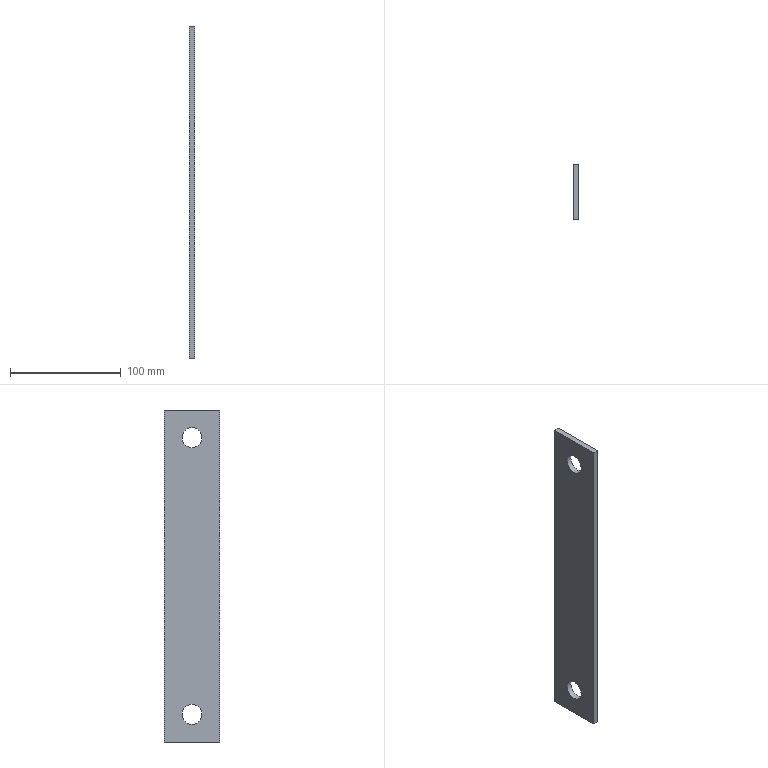Part | NX | features solid 2 | 1 solid | 8 faces | box 5 x 50 x 300 mm | volume 72455 mm3 | plane 6 | cylinder 2 | commonest cylinder face diameters 18 x2
STEP:
#1=CARTESIAN_POINT('',(700.,395.,165.));
#2=VERTEX_POINT('',#1);
#3=CARTESIAN_POINT('',(705.,395.,165.));
#4=VERTEX_POINT('',#3);
#5=CARTESIAN_POINT('',(690.,395.,165.));
#6=DIRECTION('',(1.,0.,0.));
#7=VECTOR('',#6,1000.);
#8=LINE('',#5,#7);
#9=EDGE_CURVE('',#2,#4,#8,.T.);
#10=ORIENTED_EDGE('',*,*,#9,.F.);
#11=CARTESIAN_POINT('',(700.,345.,165.));
#12=VERTEX_POINT('',#11);
#13=CARTESIAN_POINT('',(700.,350.,165.));
#14=DIRECTION('',(0.,-1.,0.));
#15=VECTOR('',#14,1000.);
#16=LINE('',#13,#15);
#17=EDGE_CURVE('',#12,#2,#16,.F.);
#18=ORIENTED_EDGE('',*,*,#17,.F.);
#19=CARTESIAN_POINT('',(705.,345.,165.));
#20=VERTEX_POINT('',#19);
#21=CARTESIAN_POINT('',(700.,345.,165.));
#22=DIRECTION('',(-1.,0.,0.));
#23=VECTOR('',#22,1000.);
#24=LINE('',#21,#23);
#25=EDGE_CURVE('',#12,#20,#24,.F.);
#26=ORIENTED_EDGE('',*,*,#25,.T.);
#27=CARTESIAN_POINT('',(705.,350.,165.));
#28=DIRECTION('',(0.,-1.,0.));
#29=VECTOR('',#28,1000.);
#30=LINE('',#27,#29);
#31=EDGE_CURVE('',#20,#4,#30,.F.);
#32=ORIENTED_EDGE('',*,*,#31,.T.);
#33=EDGE_LOOP('',(#10,#18,#26,#32));
#34=FACE_BOUND('',#33,.T.);
#35=CARTESIAN_POINT('',(690.,350.,165.));
#36=DIRECTION('',(0.,0.,1.));
#37=DIRECTION('',(0.,1.,0.));
#38=AXIS2_PLACEMENT_3D('',#35,#36,#37);
#39=PLANE('',#38);
#40=ADVANCED_FACE('',(#34),#39,.T.);
#41=ORIENTED_EDGE('',*,*,#25,.F.);
#42=CARTESIAN_POINT('',(700.,345.,-135.));
#43=VERTEX_POINT('',#42);
#44=CARTESIAN_POINT('',(700.,345.,-35.));
#45=DIRECTION('',(0.,0.,-1.));
#46=VECTOR('',#45,1000.);
#47=LINE('',#44,#46);
#48=EDGE_CURVE('',#12,#43,#47,.T.);
#49=ORIENTED_EDGE('',*,*,#48,.T.);
#50=CARTESIAN_POINT('',(705.,345.,-135.));
#51=VERTEX_POINT('',#50);
#52=CARTESIAN_POINT('',(700.,345.,-135.));
#53=DIRECTION('',(-1.,0.,0.));
#54=VECTOR('',#53,1000.);
#55=LINE('',#52,#54);
#56=EDGE_CURVE('',#43,#51,#55,.F.);
#57=ORIENTED_EDGE('',*,*,#56,.T.);
#58=CARTESIAN_POINT('',(705.,345.,-35.));
#59=DIRECTION('',(0.,0.,1.));
#60=VECTOR('',#59,1000.);
#61=LINE('',#58,#60);
#62=EDGE_CURVE('',#20,#51,#61,.F.);
#63=ORIENTED_EDGE('',*,*,#62,.F.);
#64=EDGE_LOOP('',(#41,#49,#57,#63));
#65=FACE_BOUND('',#64,.T.);
#66=CARTESIAN_POINT('',(700.,345.,-35.));
#67=DIRECTION('',(0.,1.,0.));
#68=DIRECTION('',(0.,0.,-1.));
#69=AXIS2_PLACEMENT_3D('',#66,#67,#68);
#70=PLANE('',#69);
#71=ADVANCED_FACE('',(#65),#70,.F.);
#72=ORIENTED_EDGE('',*,*,#56,.F.);
#73=CARTESIAN_POINT('',(700.,395.,-135.));
#74=VERTEX_POINT('',#73);
#75=CARTESIAN_POINT('',(700.,345.,-135.));
#76=DIRECTION('',(0.,1.,0.));
#77=VECTOR('',#76,1000.);
#78=LINE('',#75,#77);
#79=EDGE_CURVE('',#43,#74,#78,.T.);
#80=ORIENTED_EDGE('',*,*,#79,.T.);
#81=CARTESIAN_POINT('',(705.,395.,-135.));
#82=VERTEX_POINT('',#81);
#83=CARTESIAN_POINT('',(700.,395.,-135.));
#84=DIRECTION('',(-1.,0.,0.));
#85=VECTOR('',#84,1000.);
#86=LINE('',#83,#85);
#87=EDGE_CURVE('',#74,#82,#86,.F.);
#88=ORIENTED_EDGE('',*,*,#87,.T.);
#89=CARTESIAN_POINT('',(705.,345.,-135.));
#90=DIRECTION('',(0.,1.,0.));
#91=VECTOR('',#90,1000.);
#92=LINE('',#89,#91);
#93=EDGE_CURVE('',#51,#82,#92,.T.);
#94=ORIENTED_EDGE('',*,*,#93,.F.);
#95=EDGE_LOOP('',(#72,#80,#88,#94));
#96=FACE_BOUND('',#95,.T.);
#97=CARTESIAN_POINT('',(700.,345.,-135.));
#98=DIRECTION('',(0.,0.,1.));
#99=DIRECTION('',(0.,1.,0.));
#100=AXIS2_PLACEMENT_3D('',#97,#98,#99);
#101=PLANE('',#100);
#102=ADVANCED_FACE('',(#96),#101,.F.);
#103=CARTESIAN_POINT('',(700.,395.,-35.));
#104=DIRECTION('',(0.,0.,-1.));
#105=VECTOR('',#104,1000.);
#106=LINE('',#103,#105);
#107=EDGE_CURVE('',#2,#74,#106,.T.);
#108=ORIENTED_EDGE('',*,*,#107,.F.);
#109=ORIENTED_EDGE('',*,*,#9,.T.);
#110=CARTESIAN_POINT('',(705.,395.,-35.));
#111=DIRECTION('',(0.,0.,1.));
#112=VECTOR('',#111,1000.);
#113=LINE('',#110,#112);
#114=EDGE_CURVE('',#4,#82,#113,.F.);
#115=ORIENTED_EDGE('',*,*,#114,.T.);
#116=ORIENTED_EDGE('',*,*,#87,.F.);
#117=EDGE_LOOP('',(#108,#109,#115,#116));
#118=FACE_BOUND('',#117,.T.);
#119=CARTESIAN_POINT('',(700.,395.,-35.));
#120=DIRECTION('',(0.,1.,0.));
#121=DIRECTION('',(0.,0.,-1.));
#122=AXIS2_PLACEMENT_3D('',#119,#120,#121);
#123=PLANE('',#122);
#124=ADVANCED_FACE('',(#118),#123,.T.);
#125=CARTESIAN_POINT('',(705.,370.,131.));
#126=VERTEX_POINT('',#125);
#127=CARTESIAN_POINT('',(705.,370.,140.));
#128=DIRECTION('',(1.,0.,0.));
#129=DIRECTION('',(0.,0.,-1.));
#130=AXIS2_PLACEMENT_3D('',#127,#128,#129);
#131=CIRCLE('',#130,9.);
#132=EDGE_CURVE('',#126,#126,#131,.T.);
#133=ORIENTED_EDGE('',*,*,#132,.F.);
#134=EDGE_LOOP('',(#133));
#135=FACE_BOUND('',#134,.T.);
#136=CARTESIAN_POINT('',(705.,370.,-119.));
#137=VERTEX_POINT('',#136);
#138=CARTESIAN_POINT('',(705.,370.,-110.));
#139=DIRECTION('',(1.,0.,0.));
#140=DIRECTION('',(0.,0.,-1.));
#141=AXIS2_PLACEMENT_3D('',#138,#139,#140);
#142=CIRCLE('',#141,9.);
#143=EDGE_CURVE('',#137,#137,#142,.T.);
#144=ORIENTED_EDGE('',*,*,#143,.F.);
#145=EDGE_LOOP('',(#144));
#146=FACE_BOUND('',#145,.T.);
#147=ORIENTED_EDGE('',*,*,#93,.T.);
#148=ORIENTED_EDGE('',*,*,#114,.F.);
#149=ORIENTED_EDGE('',*,*,#31,.F.);
#150=ORIENTED_EDGE('',*,*,#62,.T.);
#151=EDGE_LOOP('',(#147,#148,#149,#150));
#152=FACE_BOUND('',#151,.T.);
#153=CARTESIAN_POINT('',(705.,345.,-35.));
#154=DIRECTION('',(1.,0.,0.));
#155=DIRECTION('',(0.,0.,1.));
#156=AXIS2_PLACEMENT_3D('',#153,#154,#155);
#157=PLANE('',#156);
#158=ADVANCED_FACE('',(#135,#146,#152),#157,.T.);
#159=CARTESIAN_POINT('',(700.,370.,149.));
#160=VERTEX_POINT('',#159);
#161=CARTESIAN_POINT('',(700.,370.,140.));
#162=DIRECTION('',(-1.,0.,0.));
#163=DIRECTION('',(0.,0.,1.));
#164=AXIS2_PLACEMENT_3D('',#161,#162,#163);
#165=CIRCLE('',#164,9.);
#166=EDGE_CURVE('',#160,#160,#165,.T.);
#167=ORIENTED_EDGE('',*,*,#166,.F.);
#168=EDGE_LOOP('',(#167));
#169=FACE_BOUND('',#168,.T.);
#170=CARTESIAN_POINT('',(700.,370.,-101.));
#171=VERTEX_POINT('',#170);
#172=CARTESIAN_POINT('',(700.,370.,-110.));
#173=DIRECTION('',(-1.,0.,0.));
#174=DIRECTION('',(0.,0.,1.));
#175=AXIS2_PLACEMENT_3D('',#172,#173,#174);
#176=CIRCLE('',#175,9.);
#177=EDGE_CURVE('',#171,#171,#176,.T.);
#178=ORIENTED_EDGE('',*,*,#177,.F.);
#179=EDGE_LOOP('',(#178));
#180=FACE_BOUND('',#179,.T.);
#181=ORIENTED_EDGE('',*,*,#79,.F.);
#182=ORIENTED_EDGE('',*,*,#48,.F.);
#183=ORIENTED_EDGE('',*,*,#17,.T.);
#184=ORIENTED_EDGE('',*,*,#107,.T.);
#185=EDGE_LOOP('',(#181,#182,#183,#184));
#186=FACE_BOUND('',#185,.T.);
#187=CARTESIAN_POINT('',(700.,345.,-35.));
#188=DIRECTION('',(1.,0.,0.));
#189=DIRECTION('',(0.,0.,1.));
#190=AXIS2_PLACEMENT_3D('',#187,#188,#189);
#191=PLANE('',#190);
#192=ADVANCED_FACE('',(#169,#180,#186),#191,.F.);
#193=ORIENTED_EDGE('',*,*,#143,.T.);
#194=EDGE_LOOP('',(#193));
#195=FACE_BOUND('',#194,.T.);
#196=ORIENTED_EDGE('',*,*,#177,.T.);
#197=EDGE_LOOP('',(#196));
#198=FACE_BOUND('',#197,.T.);
#199=CARTESIAN_POINT('',(705.,370.,-110.));
#200=DIRECTION('',(-1.,0.,0.));
#201=DIRECTION('',(0.,0.,-1.));
#202=AXIS2_PLACEMENT_3D('',#199,#200,#201);
#203=CYLINDRICAL_SURFACE('',#202,9.);
#204=ADVANCED_FACE('',(#195,#198),#203,.F.);
#205=ORIENTED_EDGE('',*,*,#132,.T.);
#206=EDGE_LOOP('',(#205));
#207=FACE_BOUND('',#206,.T.);
#208=ORIENTED_EDGE('',*,*,#166,.T.);
#209=EDGE_LOOP('',(#208));
#210=FACE_BOUND('',#209,.T.);
#211=CARTESIAN_POINT('',(705.,370.,140.));
#212=DIRECTION('',(-1.,0.,0.));
#213=DIRECTION('',(0.,0.,-1.));
#214=AXIS2_PLACEMENT_3D('',#211,#212,#213);
#215=CYLINDRICAL_SURFACE('',#214,9.);
#216=ADVANCED_FACE('',(#207,#210),#215,.F.);
#217=CLOSED_SHELL('',(#40,#71,#102,#124,#158,#192,#204,#216));
#218=MANIFOLD_SOLID_BREP('',#217);
#219=(LENGTH_UNIT()NAMED_UNIT(*)SI_UNIT(.MILLI.,.METRE.));
#220=UNCERTAINTY_MEASURE_WITH_UNIT(LENGTH_MEASURE(0.00001),#219,'','');
#221=(NAMED_UNIT(*)PLANE_ANGLE_UNIT()SI_UNIT($,.RADIAN.));
#222=(NAMED_UNIT(*)SI_UNIT($,.STERADIAN.)SOLID_ANGLE_UNIT());
#223=(GEOMETRIC_REPRESENTATION_CONTEXT(3)GLOBAL_UNCERTAINTY_ASSIGNED_CONTEXT((#220))GLOBAL_UNIT_ASSIGNED_CONTEXT((#219,#221,#222))REPRESENTATION_CONTEXT('',''));
#224=ADVANCED_BREP_SHAPE_REPRESENTATION('',(#218),#223);